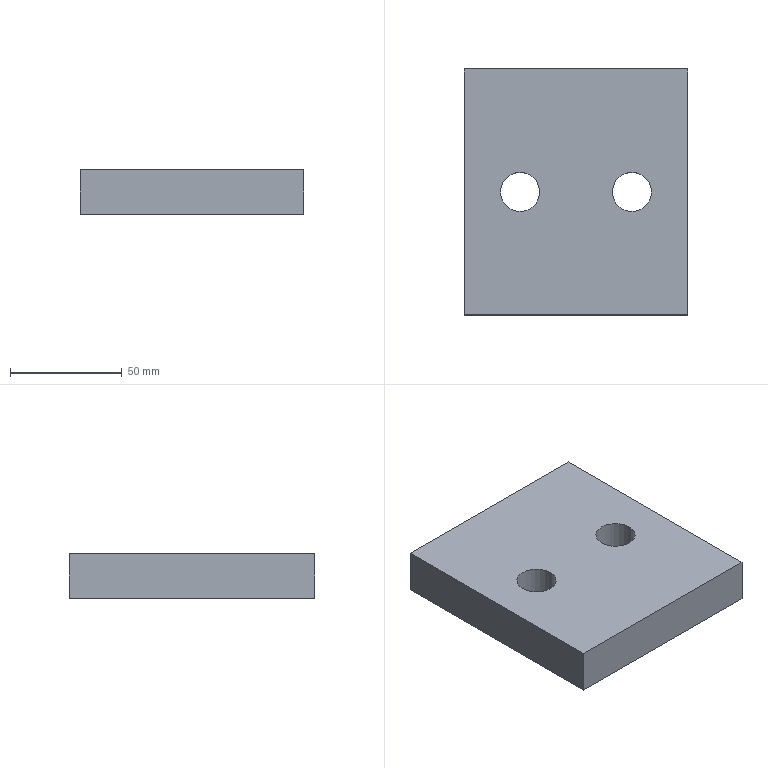Part | NX | features solid 2 | 1 solid | 8 faces | box 100 x 110 x 20 mm | volume 210379 mm3 | plane 6 | cylinder 2 | commonest cylinder face diameters 17.5 x2
STEP:
#1=CARTESIAN_POINT('',(-165.,-100.,270.));
#2=VERTEX_POINT('',#1);
#3=CARTESIAN_POINT('',(-165.,10.,270.));
#4=VERTEX_POINT('',#3);
#5=CARTESIAN_POINT('',(-165.,-69.,270.));
#6=DIRECTION('',(0.,-1.,0.));
#7=VECTOR('',#6,1000.);
#8=LINE('',#5,#7);
#9=EDGE_CURVE('',#2,#4,#8,.F.);
#10=ORIENTED_EDGE('',*,*,#9,.T.);
#11=CARTESIAN_POINT('',(-165.,10.,290.));
#12=VERTEX_POINT('',#11);
#13=CARTESIAN_POINT('',(-165.,10.,290.));
#14=DIRECTION('',(0.,0.,-1.));
#15=VECTOR('',#14,1000.);
#16=LINE('',#13,#15);
#17=EDGE_CURVE('',#12,#4,#16,.T.);
#18=ORIENTED_EDGE('',*,*,#17,.F.);
#19=CARTESIAN_POINT('',(-165.,-100.,290.));
#20=VERTEX_POINT('',#19);
#21=CARTESIAN_POINT('',(-165.,-69.,290.));
#22=DIRECTION('',(0.,-1.,0.));
#23=VECTOR('',#22,1000.);
#24=LINE('',#21,#23);
#25=EDGE_CURVE('',#20,#12,#24,.F.);
#26=ORIENTED_EDGE('',*,*,#25,.F.);
#27=CARTESIAN_POINT('',(-165.,-100.,290.));
#28=DIRECTION('',(0.,0.,-1.));
#29=VECTOR('',#28,1000.);
#30=LINE('',#27,#29);
#31=EDGE_CURVE('',#20,#2,#30,.T.);
#32=ORIENTED_EDGE('',*,*,#31,.T.);
#33=EDGE_LOOP('',(#10,#18,#26,#32));
#34=FACE_BOUND('',#33,.T.);
#35=CARTESIAN_POINT('',(-165.,-69.,290.));
#36=DIRECTION('',(-1.,0.,0.));
#37=DIRECTION('',(0.,0.,1.));
#38=AXIS2_PLACEMENT_3D('',#35,#36,#37);
#39=PLANE('',#38);
#40=ADVANCED_FACE('',(#34),#39,.F.);
#41=CARTESIAN_POINT('',(-265.,10.,270.));
#42=VERTEX_POINT('',#41);
#43=CARTESIAN_POINT('',(-265.,10.,270.));
#44=DIRECTION('',(1.,0.,0.));
#45=VECTOR('',#44,1000.);
#46=LINE('',#43,#45);
#47=EDGE_CURVE('',#42,#4,#46,.T.);
#48=ORIENTED_EDGE('',*,*,#47,.F.);
#49=CARTESIAN_POINT('',(-265.,10.,290.));
#50=VERTEX_POINT('',#49);
#51=CARTESIAN_POINT('',(-265.,10.,290.));
#52=DIRECTION('',(0.,0.,-1.));
#53=VECTOR('',#52,1000.);
#54=LINE('',#51,#53);
#55=EDGE_CURVE('',#50,#42,#54,.T.);
#56=ORIENTED_EDGE('',*,*,#55,.F.);
#57=CARTESIAN_POINT('',(-265.,10.,290.));
#58=DIRECTION('',(1.,0.,0.));
#59=VECTOR('',#58,1000.);
#60=LINE('',#57,#59);
#61=EDGE_CURVE('',#50,#12,#60,.T.);
#62=ORIENTED_EDGE('',*,*,#61,.T.);
#63=ORIENTED_EDGE('',*,*,#17,.T.);
#64=EDGE_LOOP('',(#48,#56,#62,#63));
#65=FACE_BOUND('',#64,.T.);
#66=CARTESIAN_POINT('',(-265.,10.,190.));
#67=DIRECTION('',(0.,1.,0.));
#68=DIRECTION('',(1.,0.,0.));
#69=AXIS2_PLACEMENT_3D('',#66,#67,#68);
#70=PLANE('',#69);
#71=ADVANCED_FACE('',(#65),#70,.T.);
#72=CARTESIAN_POINT('',(-265.,-100.,270.));
#73=VERTEX_POINT('',#72);
#74=CARTESIAN_POINT('',(-265.,-69.,270.));
#75=DIRECTION('',(0.,-1.,0.));
#76=VECTOR('',#75,1000.);
#77=LINE('',#74,#76);
#78=EDGE_CURVE('',#73,#42,#77,.F.);
#79=ORIENTED_EDGE('',*,*,#78,.F.);
#80=CARTESIAN_POINT('',(-265.,-100.,290.));
#81=VERTEX_POINT('',#80);
#82=CARTESIAN_POINT('',(-265.,-100.,290.));
#83=DIRECTION('',(0.,0.,-1.));
#84=VECTOR('',#83,1000.);
#85=LINE('',#82,#84);
#86=EDGE_CURVE('',#81,#73,#85,.T.);
#87=ORIENTED_EDGE('',*,*,#86,.F.);
#88=CARTESIAN_POINT('',(-265.,-69.,290.));
#89=DIRECTION('',(0.,-1.,0.));
#90=VECTOR('',#89,1000.);
#91=LINE('',#88,#90);
#92=EDGE_CURVE('',#81,#50,#91,.F.);
#93=ORIENTED_EDGE('',*,*,#92,.T.);
#94=ORIENTED_EDGE('',*,*,#55,.T.);
#95=EDGE_LOOP('',(#79,#87,#93,#94));
#96=FACE_BOUND('',#95,.T.);
#97=CARTESIAN_POINT('',(-265.,-69.,290.));
#98=DIRECTION('',(-1.,0.,0.));
#99=DIRECTION('',(0.,0.,1.));
#100=AXIS2_PLACEMENT_3D('',#97,#98,#99);
#101=PLANE('',#100);
#102=ADVANCED_FACE('',(#96),#101,.T.);
#103=CARTESIAN_POINT('',(-265.,-100.,270.));
#104=DIRECTION('',(1.,0.,0.));
#105=VECTOR('',#104,1000.);
#106=LINE('',#103,#105);
#107=EDGE_CURVE('',#73,#2,#106,.T.);
#108=ORIENTED_EDGE('',*,*,#107,.T.);
#109=ORIENTED_EDGE('',*,*,#31,.F.);
#110=CARTESIAN_POINT('',(-265.,-100.,290.));
#111=DIRECTION('',(1.,0.,0.));
#112=VECTOR('',#111,1000.);
#113=LINE('',#110,#112);
#114=EDGE_CURVE('',#81,#20,#113,.T.);
#115=ORIENTED_EDGE('',*,*,#114,.F.);
#116=ORIENTED_EDGE('',*,*,#86,.T.);
#117=EDGE_LOOP('',(#108,#109,#115,#116));
#118=FACE_BOUND('',#117,.T.);
#119=CARTESIAN_POINT('',(-265.,-100.,190.));
#120=DIRECTION('',(0.,1.,0.));
#121=DIRECTION('',(1.,0.,0.));
#122=AXIS2_PLACEMENT_3D('',#119,#120,#121);
#123=PLANE('',#122);
#124=ADVANCED_FACE('',(#118),#123,.F.);
#125=CARTESIAN_POINT('',(-190.,-53.75,290.));
#126=VERTEX_POINT('',#125);
#127=CARTESIAN_POINT('',(-190.,-45.,290.));
#128=DIRECTION('',(0.,0.,-1.));
#129=DIRECTION('',(0.,-1.,0.));
#130=AXIS2_PLACEMENT_3D('',#127,#128,#129);
#131=CIRCLE('',#130,8.75);
#132=EDGE_CURVE('',#126,#126,#131,.T.);
#133=ORIENTED_EDGE('',*,*,#132,.T.);
#134=EDGE_LOOP('',(#133));
#135=FACE_BOUND('',#134,.T.);
#136=CARTESIAN_POINT('',(-240.,-53.75,290.));
#137=VERTEX_POINT('',#136);
#138=CARTESIAN_POINT('',(-240.,-45.,290.));
#139=DIRECTION('',(0.,0.,-1.));
#140=DIRECTION('',(0.,-1.,0.));
#141=AXIS2_PLACEMENT_3D('',#138,#139,#140);
#142=CIRCLE('',#141,8.75);
#143=EDGE_CURVE('',#137,#137,#142,.T.);
#144=ORIENTED_EDGE('',*,*,#143,.T.);
#145=EDGE_LOOP('',(#144));
#146=FACE_BOUND('',#145,.T.);
#147=ORIENTED_EDGE('',*,*,#25,.T.);
#148=ORIENTED_EDGE('',*,*,#61,.F.);
#149=ORIENTED_EDGE('',*,*,#92,.F.);
#150=ORIENTED_EDGE('',*,*,#114,.T.);
#151=EDGE_LOOP('',(#147,#148,#149,#150));
#152=FACE_BOUND('',#151,.T.);
#153=CARTESIAN_POINT('',(-265.,-69.,290.));
#154=DIRECTION('',(0.,0.,-1.));
#155=DIRECTION('',(0.,-1.,0.));
#156=AXIS2_PLACEMENT_3D('',#153,#154,#155);
#157=PLANE('',#156);
#158=ADVANCED_FACE('',(#135,#146,#152),#157,.F.);
#159=CARTESIAN_POINT('',(-190.,-53.75,270.));
#160=VERTEX_POINT('',#159);
#161=CARTESIAN_POINT('',(-190.,-45.,270.));
#162=DIRECTION('',(0.,0.,-1.));
#163=DIRECTION('',(0.,-1.,0.));
#164=AXIS2_PLACEMENT_3D('',#161,#162,#163);
#165=CIRCLE('',#164,8.75);
#166=EDGE_CURVE('',#160,#160,#165,.T.);
#167=ORIENTED_EDGE('',*,*,#166,.F.);
#168=EDGE_LOOP('',(#167));
#169=FACE_BOUND('',#168,.T.);
#170=CARTESIAN_POINT('',(-240.,-53.75,270.));
#171=VERTEX_POINT('',#170);
#172=CARTESIAN_POINT('',(-240.,-45.,270.));
#173=DIRECTION('',(0.,0.,-1.));
#174=DIRECTION('',(0.,-1.,0.));
#175=AXIS2_PLACEMENT_3D('',#172,#173,#174);
#176=CIRCLE('',#175,8.75);
#177=EDGE_CURVE('',#171,#171,#176,.T.);
#178=ORIENTED_EDGE('',*,*,#177,.F.);
#179=EDGE_LOOP('',(#178));
#180=FACE_BOUND('',#179,.T.);
#181=ORIENTED_EDGE('',*,*,#9,.F.);
#182=ORIENTED_EDGE('',*,*,#107,.F.);
#183=ORIENTED_EDGE('',*,*,#78,.T.);
#184=ORIENTED_EDGE('',*,*,#47,.T.);
#185=EDGE_LOOP('',(#181,#182,#183,#184));
#186=FACE_BOUND('',#185,.T.);
#187=CARTESIAN_POINT('',(-265.,-69.,270.));
#188=DIRECTION('',(0.,0.,-1.));
#189=DIRECTION('',(0.,-1.,0.));
#190=AXIS2_PLACEMENT_3D('',#187,#188,#189);
#191=PLANE('',#190);
#192=ADVANCED_FACE('',(#169,#180,#186),#191,.T.);
#193=ORIENTED_EDGE('',*,*,#177,.T.);
#194=EDGE_LOOP('',(#193));
#195=FACE_BOUND('',#194,.T.);
#196=ORIENTED_EDGE('',*,*,#143,.F.);
#197=EDGE_LOOP('',(#196));
#198=FACE_BOUND('',#197,.T.);
#199=CARTESIAN_POINT('',(-240.,-45.,290.));
#200=DIRECTION('',(0.,0.,-1.));
#201=DIRECTION('',(0.,-1.,0.));
#202=AXIS2_PLACEMENT_3D('',#199,#200,#201);
#203=CYLINDRICAL_SURFACE('',#202,8.75);
#204=ADVANCED_FACE('',(#195,#198),#203,.F.);
#205=ORIENTED_EDGE('',*,*,#166,.T.);
#206=EDGE_LOOP('',(#205));
#207=FACE_BOUND('',#206,.T.);
#208=ORIENTED_EDGE('',*,*,#132,.F.);
#209=EDGE_LOOP('',(#208));
#210=FACE_BOUND('',#209,.T.);
#211=CARTESIAN_POINT('',(-190.,-45.,290.));
#212=DIRECTION('',(0.,0.,-1.));
#213=DIRECTION('',(0.,-1.,0.));
#214=AXIS2_PLACEMENT_3D('',#211,#212,#213);
#215=CYLINDRICAL_SURFACE('',#214,8.75);
#216=ADVANCED_FACE('',(#207,#210),#215,.F.);
#217=CLOSED_SHELL('',(#40,#71,#102,#124,#158,#192,#204,#216));
#218=MANIFOLD_SOLID_BREP('',#217);
#219=(LENGTH_UNIT()NAMED_UNIT(*)SI_UNIT(.MILLI.,.METRE.));
#220=UNCERTAINTY_MEASURE_WITH_UNIT(LENGTH_MEASURE(0.00001),#219,'','');
#221=(NAMED_UNIT(*)PLANE_ANGLE_UNIT()SI_UNIT($,.RADIAN.));
#222=(NAMED_UNIT(*)SI_UNIT($,.STERADIAN.)SOLID_ANGLE_UNIT());
#223=(GEOMETRIC_REPRESENTATION_CONTEXT(3)GLOBAL_UNCERTAINTY_ASSIGNED_CONTEXT((#220))GLOBAL_UNIT_ASSIGNED_CONTEXT((#219,#221,#222))REPRESENTATION_CONTEXT('',''));
#224=ADVANCED_BREP_SHAPE_REPRESENTATION('',(#218),#223);